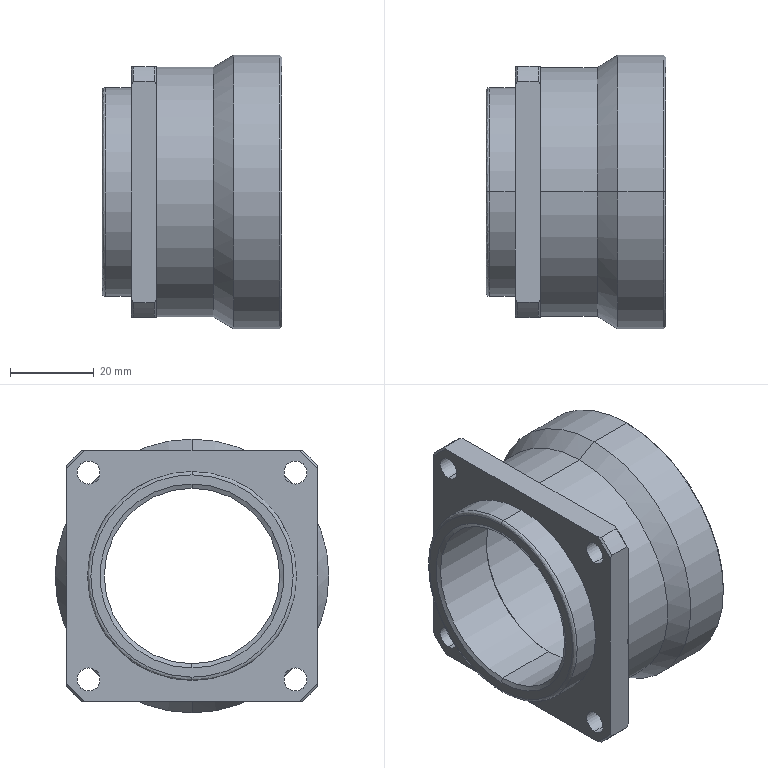Part | STEP file | _X2_8f9351fa51859f7f5708_X0_MFB060_5.STEP.STEP | 1 solid | 56 faces | box 43 x 65.5 x 65.5 mm | volume 50980 mm3 | cylinder 24 | cone 16 | plane 10 | spline 6 | commonest cylinder face diameters 5.5 x8 50 x4 80 x4 42 x2 52 x2 59.8 x2